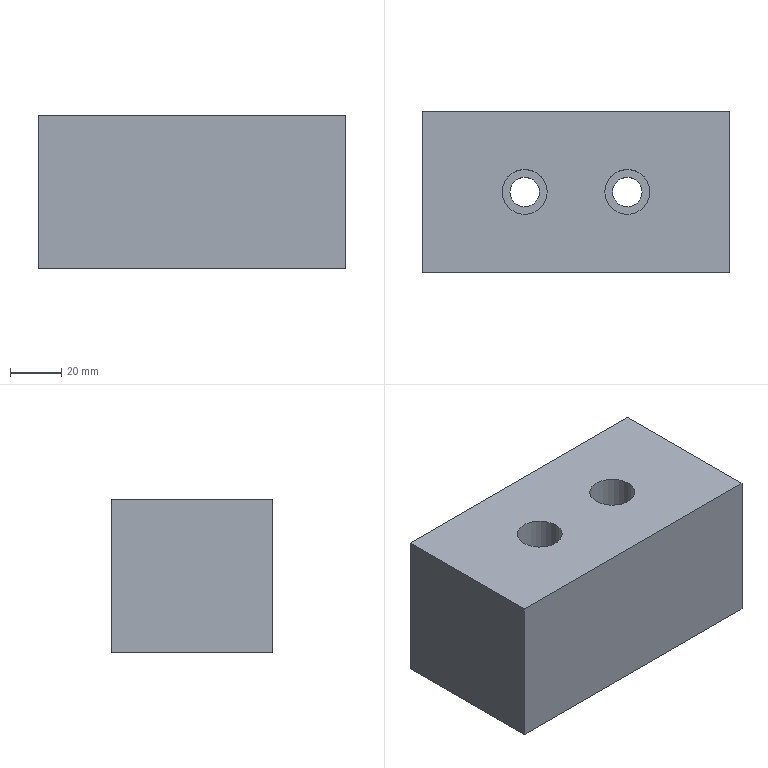Part | NX | features solid 2 | 1 solid | 12 faces | box 120 x 63 x 60 mm | volume 430203 mm3 | plane 8 | cylinder 4 | commonest cylinder face diameters 11.5 x2 17.5 x2
STEP:
#1=CARTESIAN_POINT('',(-645.,162.,120.));
#2=VERTEX_POINT('',#1);
#3=CARTESIAN_POINT('',(-765.,162.,120.));
#4=VERTEX_POINT('',#3);
#5=CARTESIAN_POINT('',(-630.,162.,120.));
#6=DIRECTION('',(-1.,0.,0.));
#7=VECTOR('',#6,1000.);
#8=LINE('',#5,#7);
#9=EDGE_CURVE('',#2,#4,#8,.T.);
#10=ORIENTED_EDGE('',*,*,#9,.T.);
#11=CARTESIAN_POINT('',(-765.,162.,60.));
#12=VERTEX_POINT('',#11);
#13=CARTESIAN_POINT('',(-765.,162.,60.));
#14=DIRECTION('',(0.,0.,1.));
#15=VECTOR('',#14,1000.);
#16=LINE('',#13,#15);
#17=EDGE_CURVE('',#12,#4,#16,.T.);
#18=ORIENTED_EDGE('',*,*,#17,.F.);
#19=CARTESIAN_POINT('',(-645.,162.,60.));
#20=VERTEX_POINT('',#19);
#21=CARTESIAN_POINT('',(-630.,162.,60.));
#22=DIRECTION('',(-1.,0.,0.));
#23=VECTOR('',#22,1000.);
#24=LINE('',#21,#23);
#25=EDGE_CURVE('',#20,#12,#24,.T.);
#26=ORIENTED_EDGE('',*,*,#25,.F.);
#27=CARTESIAN_POINT('',(-645.,162.,60.));
#28=DIRECTION('',(0.,0.,1.));
#29=VECTOR('',#28,1000.);
#30=LINE('',#27,#29);
#31=EDGE_CURVE('',#20,#2,#30,.T.);
#32=ORIENTED_EDGE('',*,*,#31,.T.);
#33=EDGE_LOOP('',(#10,#18,#26,#32));
#34=FACE_BOUND('',#33,.T.);
#35=CARTESIAN_POINT('',(-630.,162.,60.));
#36=DIRECTION('',(0.,-1.,0.));
#37=DIRECTION('',(0.,0.,1.));
#38=AXIS2_PLACEMENT_3D('',#35,#36,#37);
#39=PLANE('',#38);
#40=ADVANCED_FACE('',(#34),#39,.T.);
#41=CARTESIAN_POINT('',(-765.,225.,120.));
#42=VERTEX_POINT('',#41);
#43=CARTESIAN_POINT('',(-765.,238.5,120.));
#44=DIRECTION('',(0.,-1.,0.));
#45=VECTOR('',#44,1000.);
#46=LINE('',#43,#45);
#47=EDGE_CURVE('',#42,#4,#46,.T.);
#48=ORIENTED_EDGE('',*,*,#47,.F.);
#49=CARTESIAN_POINT('',(-765.,225.,60.));
#50=VERTEX_POINT('',#49);
#51=CARTESIAN_POINT('',(-765.,225.,60.));
#52=DIRECTION('',(0.,0.,1.));
#53=VECTOR('',#52,1000.);
#54=LINE('',#51,#53);
#55=EDGE_CURVE('',#50,#42,#54,.T.);
#56=ORIENTED_EDGE('',*,*,#55,.F.);
#57=CARTESIAN_POINT('',(-765.,238.5,60.));
#58=DIRECTION('',(0.,-1.,0.));
#59=VECTOR('',#58,1000.);
#60=LINE('',#57,#59);
#61=EDGE_CURVE('',#50,#12,#60,.T.);
#62=ORIENTED_EDGE('',*,*,#61,.T.);
#63=ORIENTED_EDGE('',*,*,#17,.T.);
#64=EDGE_LOOP('',(#48,#56,#62,#63));
#65=FACE_BOUND('',#64,.T.);
#66=CARTESIAN_POINT('',(-765.,238.5,60.));
#67=DIRECTION('',(1.,0.,0.));
#68=DIRECTION('',(0.,0.,-1.));
#69=AXIS2_PLACEMENT_3D('',#66,#67,#68);
#70=PLANE('',#69);
#71=ADVANCED_FACE('',(#65),#70,.F.);
#72=CARTESIAN_POINT('',(-645.,225.,120.));
#73=VERTEX_POINT('',#72);
#74=CARTESIAN_POINT('',(-630.,225.,120.));
#75=DIRECTION('',(-1.,0.,0.));
#76=VECTOR('',#75,1000.);
#77=LINE('',#74,#76);
#78=EDGE_CURVE('',#73,#42,#77,.T.);
#79=ORIENTED_EDGE('',*,*,#78,.F.);
#80=CARTESIAN_POINT('',(-645.,225.,60.));
#81=VERTEX_POINT('',#80);
#82=CARTESIAN_POINT('',(-645.,225.,60.));
#83=DIRECTION('',(0.,0.,1.));
#84=VECTOR('',#83,1000.);
#85=LINE('',#82,#84);
#86=EDGE_CURVE('',#81,#73,#85,.T.);
#87=ORIENTED_EDGE('',*,*,#86,.F.);
#88=CARTESIAN_POINT('',(-630.,225.,60.));
#89=DIRECTION('',(-1.,0.,0.));
#90=VECTOR('',#89,1000.);
#91=LINE('',#88,#90);
#92=EDGE_CURVE('',#81,#50,#91,.T.);
#93=ORIENTED_EDGE('',*,*,#92,.T.);
#94=ORIENTED_EDGE('',*,*,#55,.T.);
#95=EDGE_LOOP('',(#79,#87,#93,#94));
#96=FACE_BOUND('',#95,.T.);
#97=CARTESIAN_POINT('',(-630.,225.,60.));
#98=DIRECTION('',(0.,-1.,0.));
#99=DIRECTION('',(0.,0.,1.));
#100=AXIS2_PLACEMENT_3D('',#97,#98,#99);
#101=PLANE('',#100);
#102=ADVANCED_FACE('',(#96),#101,.F.);
#103=CARTESIAN_POINT('',(-645.,238.5,120.));
#104=DIRECTION('',(0.,-1.,0.));
#105=VECTOR('',#104,1000.);
#106=LINE('',#103,#105);
#107=EDGE_CURVE('',#73,#2,#106,.T.);
#108=ORIENTED_EDGE('',*,*,#107,.T.);
#109=ORIENTED_EDGE('',*,*,#31,.F.);
#110=CARTESIAN_POINT('',(-645.,238.5,60.));
#111=DIRECTION('',(0.,-1.,0.));
#112=VECTOR('',#111,1000.);
#113=LINE('',#110,#112);
#114=EDGE_CURVE('',#81,#20,#113,.T.);
#115=ORIENTED_EDGE('',*,*,#114,.F.);
#116=ORIENTED_EDGE('',*,*,#86,.T.);
#117=EDGE_LOOP('',(#108,#109,#115,#116));
#118=FACE_BOUND('',#117,.T.);
#119=CARTESIAN_POINT('',(-645.,238.5,60.));
#120=DIRECTION('',(1.,0.,0.));
#121=DIRECTION('',(0.,0.,-1.));
#122=AXIS2_PLACEMENT_3D('',#119,#120,#121);
#123=PLANE('',#122);
#124=ADVANCED_FACE('',(#118),#123,.T.);
#125=CARTESIAN_POINT('',(-730.75,193.5,60.));
#126=VERTEX_POINT('',#125);
#127=CARTESIAN_POINT('',(-725.,193.5,60.));
#128=DIRECTION('',(0.,0.,1.));
#129=DIRECTION('',(-1.,0.,0.));
#130=AXIS2_PLACEMENT_3D('',#127,#128,#129);
#131=CIRCLE('',#130,5.75);
#132=EDGE_CURVE('',#126,#126,#131,.T.);
#133=ORIENTED_EDGE('',*,*,#132,.T.);
#134=EDGE_LOOP('',(#133));
#135=FACE_BOUND('',#134,.T.);
#136=CARTESIAN_POINT('',(-690.75,193.5,60.));
#137=VERTEX_POINT('',#136);
#138=CARTESIAN_POINT('',(-685.,193.5,60.));
#139=DIRECTION('',(0.,0.,1.));
#140=DIRECTION('',(-1.,0.,0.));
#141=AXIS2_PLACEMENT_3D('',#138,#139,#140);
#142=CIRCLE('',#141,5.75);
#143=EDGE_CURVE('',#137,#137,#142,.T.);
#144=ORIENTED_EDGE('',*,*,#143,.T.);
#145=EDGE_LOOP('',(#144));
#146=FACE_BOUND('',#145,.T.);
#147=ORIENTED_EDGE('',*,*,#25,.T.);
#148=ORIENTED_EDGE('',*,*,#61,.F.);
#149=ORIENTED_EDGE('',*,*,#92,.F.);
#150=ORIENTED_EDGE('',*,*,#114,.T.);
#151=EDGE_LOOP('',(#147,#148,#149,#150));
#152=FACE_BOUND('',#151,.T.);
#153=CARTESIAN_POINT('',(-630.,238.5,60.));
#154=DIRECTION('',(0.,0.,-1.));
#155=DIRECTION('',(-1.,0.,0.));
#156=AXIS2_PLACEMENT_3D('',#153,#154,#155);
#157=PLANE('',#156);
#158=ADVANCED_FACE('',(#135,#146,#152),#157,.T.);
#159=CARTESIAN_POINT('',(-716.25,193.5,120.));
#160=VERTEX_POINT('',#159);
#161=CARTESIAN_POINT('',(-725.,193.5,120.));
#162=DIRECTION('',(0.,0.,-1.));
#163=DIRECTION('',(1.,0.,0.));
#164=AXIS2_PLACEMENT_3D('',#161,#162,#163);
#165=CIRCLE('',#164,8.75);
#166=EDGE_CURVE('',#160,#160,#165,.F.);
#167=ORIENTED_EDGE('',*,*,#166,.F.);
#168=EDGE_LOOP('',(#167));
#169=FACE_BOUND('',#168,.T.);
#170=CARTESIAN_POINT('',(-676.25,193.5,120.));
#171=VERTEX_POINT('',#170);
#172=CARTESIAN_POINT('',(-685.,193.5,120.));
#173=DIRECTION('',(0.,0.,-1.));
#174=DIRECTION('',(1.,0.,0.));
#175=AXIS2_PLACEMENT_3D('',#172,#173,#174);
#176=CIRCLE('',#175,8.75);
#177=EDGE_CURVE('',#171,#171,#176,.F.);
#178=ORIENTED_EDGE('',*,*,#177,.F.);
#179=EDGE_LOOP('',(#178));
#180=FACE_BOUND('',#179,.T.);
#181=ORIENTED_EDGE('',*,*,#9,.F.);
#182=ORIENTED_EDGE('',*,*,#107,.F.);
#183=ORIENTED_EDGE('',*,*,#78,.T.);
#184=ORIENTED_EDGE('',*,*,#47,.T.);
#185=EDGE_LOOP('',(#181,#182,#183,#184));
#186=FACE_BOUND('',#185,.T.);
#187=CARTESIAN_POINT('',(-630.,238.5,120.));
#188=DIRECTION('',(0.,0.,-1.));
#189=DIRECTION('',(-1.,0.,0.));
#190=AXIS2_PLACEMENT_3D('',#187,#188,#189);
#191=PLANE('',#190);
#192=ADVANCED_FACE('',(#169,#180,#186),#191,.F.);
#193=ORIENTED_EDGE('',*,*,#143,.F.);
#194=EDGE_LOOP('',(#193));
#195=FACE_BOUND('',#194,.T.);
#196=CARTESIAN_POINT('',(-690.75,193.5,80.));
#197=VERTEX_POINT('',#196);
#198=CARTESIAN_POINT('',(-685.,193.5,80.));
#199=DIRECTION('',(0.,0.,1.));
#200=DIRECTION('',(-1.,0.,0.));
#201=AXIS2_PLACEMENT_3D('',#198,#199,#200);
#202=CIRCLE('',#201,5.75);
#203=EDGE_CURVE('',#197,#197,#202,.T.);
#204=ORIENTED_EDGE('',*,*,#203,.T.);
#205=EDGE_LOOP('',(#204));
#206=FACE_BOUND('',#205,.T.);
#207=CARTESIAN_POINT('',(-685.,193.5,40.));
#208=DIRECTION('',(0.,0.,-1.));
#209=DIRECTION('',(-1.,0.,0.));
#210=AXIS2_PLACEMENT_3D('',#207,#208,#209);
#211=CYLINDRICAL_SURFACE('',#210,5.75);
#212=ADVANCED_FACE('',(#195,#206),#211,.F.);
#213=ORIENTED_EDGE('',*,*,#203,.F.);
#214=EDGE_LOOP('',(#213));
#215=FACE_BOUND('',#214,.T.);
#216=CARTESIAN_POINT('',(-693.75,193.5,80.));
#217=VERTEX_POINT('',#216);
#218=CARTESIAN_POINT('',(-685.,193.5,80.));
#219=DIRECTION('',(0.,0.,1.));
#220=DIRECTION('',(-1.,0.,0.));
#221=AXIS2_PLACEMENT_3D('',#218,#219,#220);
#222=CIRCLE('',#221,8.75);
#223=EDGE_CURVE('',#217,#217,#222,.T.);
#224=ORIENTED_EDGE('',*,*,#223,.T.);
#225=EDGE_LOOP('',(#224));
#226=FACE_BOUND('',#225,.T.);
#227=CARTESIAN_POINT('',(-685.,193.5,80.));
#228=DIRECTION('',(0.,0.,-1.));
#229=DIRECTION('',(-1.,0.,0.));
#230=AXIS2_PLACEMENT_3D('',#227,#228,#229);
#231=PLANE('',#230);
#232=ADVANCED_FACE('',(#215,#226),#231,.F.);
#233=ORIENTED_EDGE('',*,*,#223,.F.);
#234=EDGE_LOOP('',(#233));
#235=FACE_BOUND('',#234,.T.);
#236=ORIENTED_EDGE('',*,*,#177,.T.);
#237=EDGE_LOOP('',(#236));
#238=FACE_BOUND('',#237,.T.);
#239=CARTESIAN_POINT('',(-685.,193.5,130.));
#240=DIRECTION('',(0.,0.,-1.));
#241=DIRECTION('',(-1.,0.,0.));
#242=AXIS2_PLACEMENT_3D('',#239,#240,#241);
#243=CYLINDRICAL_SURFACE('',#242,8.75);
#244=ADVANCED_FACE('',(#235,#238),#243,.F.);
#245=ORIENTED_EDGE('',*,*,#132,.F.);
#246=EDGE_LOOP('',(#245));
#247=FACE_BOUND('',#246,.T.);
#248=CARTESIAN_POINT('',(-730.75,193.5,80.));
#249=VERTEX_POINT('',#248);
#250=CARTESIAN_POINT('',(-725.,193.5,80.));
#251=DIRECTION('',(0.,0.,1.));
#252=DIRECTION('',(-1.,0.,0.));
#253=AXIS2_PLACEMENT_3D('',#250,#251,#252);
#254=CIRCLE('',#253,5.75);
#255=EDGE_CURVE('',#249,#249,#254,.T.);
#256=ORIENTED_EDGE('',*,*,#255,.T.);
#257=EDGE_LOOP('',(#256));
#258=FACE_BOUND('',#257,.T.);
#259=CARTESIAN_POINT('',(-725.,193.5,40.));
#260=DIRECTION('',(0.,0.,-1.));
#261=DIRECTION('',(-1.,0.,0.));
#262=AXIS2_PLACEMENT_3D('',#259,#260,#261);
#263=CYLINDRICAL_SURFACE('',#262,5.75);
#264=ADVANCED_FACE('',(#247,#258),#263,.F.);
#265=ORIENTED_EDGE('',*,*,#255,.F.);
#266=EDGE_LOOP('',(#265));
#267=FACE_BOUND('',#266,.T.);
#268=CARTESIAN_POINT('',(-733.75,193.5,80.));
#269=VERTEX_POINT('',#268);
#270=CARTESIAN_POINT('',(-725.,193.5,80.));
#271=DIRECTION('',(0.,0.,1.));
#272=DIRECTION('',(-1.,0.,0.));
#273=AXIS2_PLACEMENT_3D('',#270,#271,#272);
#274=CIRCLE('',#273,8.75);
#275=EDGE_CURVE('',#269,#269,#274,.T.);
#276=ORIENTED_EDGE('',*,*,#275,.T.);
#277=EDGE_LOOP('',(#276));
#278=FACE_BOUND('',#277,.T.);
#279=CARTESIAN_POINT('',(-725.,193.5,80.));
#280=DIRECTION('',(0.,0.,-1.));
#281=DIRECTION('',(-1.,0.,0.));
#282=AXIS2_PLACEMENT_3D('',#279,#280,#281);
#283=PLANE('',#282);
#284=ADVANCED_FACE('',(#267,#278),#283,.F.);
#285=ORIENTED_EDGE('',*,*,#275,.F.);
#286=EDGE_LOOP('',(#285));
#287=FACE_BOUND('',#286,.T.);
#288=ORIENTED_EDGE('',*,*,#166,.T.);
#289=EDGE_LOOP('',(#288));
#290=FACE_BOUND('',#289,.T.);
#291=CARTESIAN_POINT('',(-725.,193.5,130.));
#292=DIRECTION('',(0.,0.,-1.));
#293=DIRECTION('',(-1.,0.,0.));
#294=AXIS2_PLACEMENT_3D('',#291,#292,#293);
#295=CYLINDRICAL_SURFACE('',#294,8.75);
#296=ADVANCED_FACE('',(#287,#290),#295,.F.);
#297=CLOSED_SHELL('',(#40,#71,#102,#124,#158,#192,#212,#232,#244,#264,#284,#296));
#298=MANIFOLD_SOLID_BREP('',#297);
#299=(LENGTH_UNIT()NAMED_UNIT(*)SI_UNIT(.MILLI.,.METRE.));
#300=UNCERTAINTY_MEASURE_WITH_UNIT(LENGTH_MEASURE(0.00001),#299,'','');
#301=(NAMED_UNIT(*)PLANE_ANGLE_UNIT()SI_UNIT($,.RADIAN.));
#302=(NAMED_UNIT(*)SI_UNIT($,.STERADIAN.)SOLID_ANGLE_UNIT());
#303=(GEOMETRIC_REPRESENTATION_CONTEXT(3)GLOBAL_UNCERTAINTY_ASSIGNED_CONTEXT((#300))GLOBAL_UNIT_ASSIGNED_CONTEXT((#299,#301,#302))REPRESENTATION_CONTEXT('',''));
#304=ADVANCED_BREP_SHAPE_REPRESENTATION('',(#298),#303);